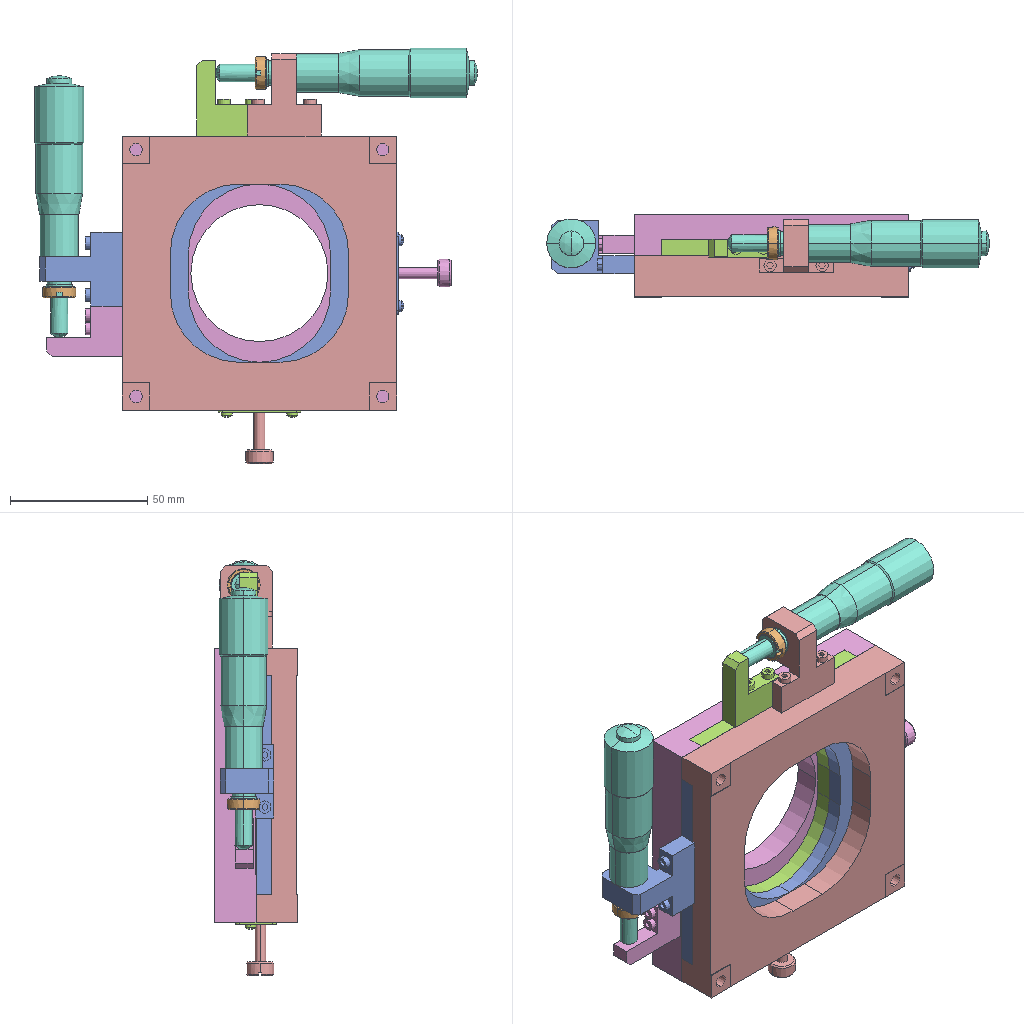Assembly | SolidWorks | 6 different items | 8 placed | box 162 x 30 x 152 mm
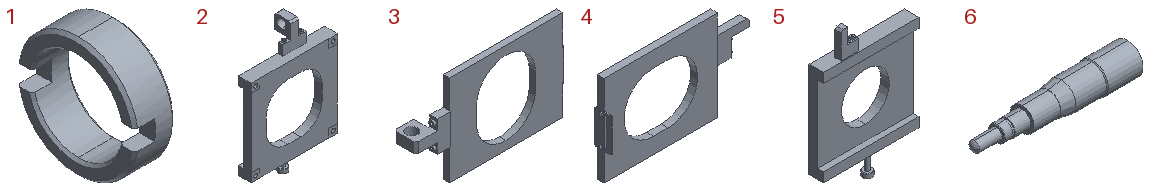Parts list (item | quantity | size | volume | features):
1 | x2 | 4 x 12 x 12 mm | 182.884 mm3 | features ICE 1, Revolution 1
2 | x1 | 100 x 28 x 149.5 mm | 72499 mm3 | features ICE 9, RevCut 4, Extrusion 1, Revolution 1
3 | x1 | 132.782 x 19.5 x 80 mm | 33329 mm3 | features ICE 10, Revolution 2, Extrusion 1
4 | x1 | 130.282 x 15 x 80 mm | 34016 mm3 | features ICE 9, Revolution 2, Extrusion 1
5 | x1 | 100 x 16 x 147.6 mm | 86306 mm3 | features RevCut 12, ICE 7, Extrusion 1, Revolution 1
6 | x2 | 95.5 x 18 x 18 mm | 15118 mm3 | features RevCut 1, Revolution 1